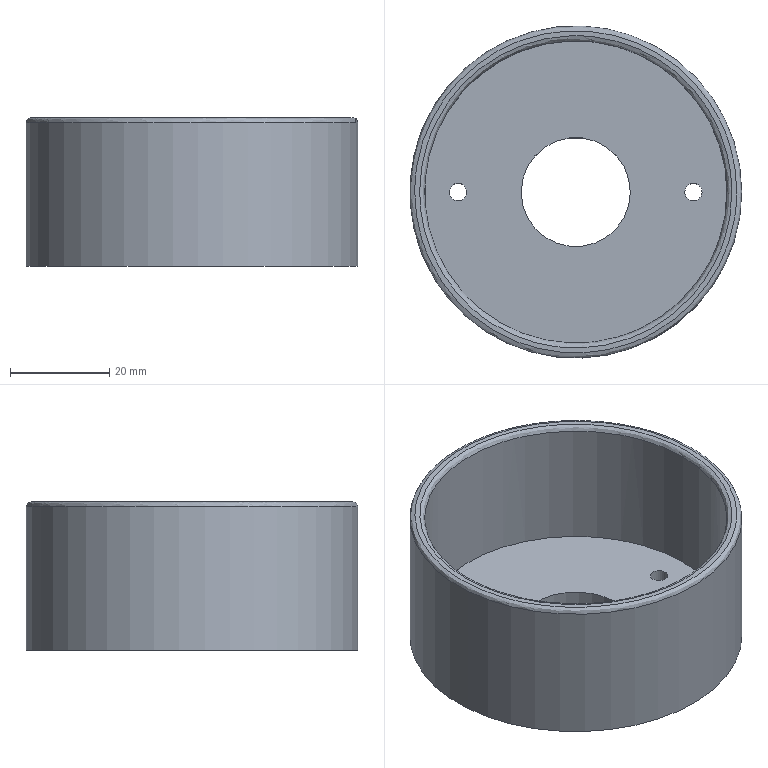Part | NX | 1 solid | 10 faces | box 67 x 67 x 30 mm | volume 25577 mm3 | cylinder 5 | plane 3 | spline 2 | commonest cylinder face diameters 3.5 x2 22 x1 61 x1 67 x1